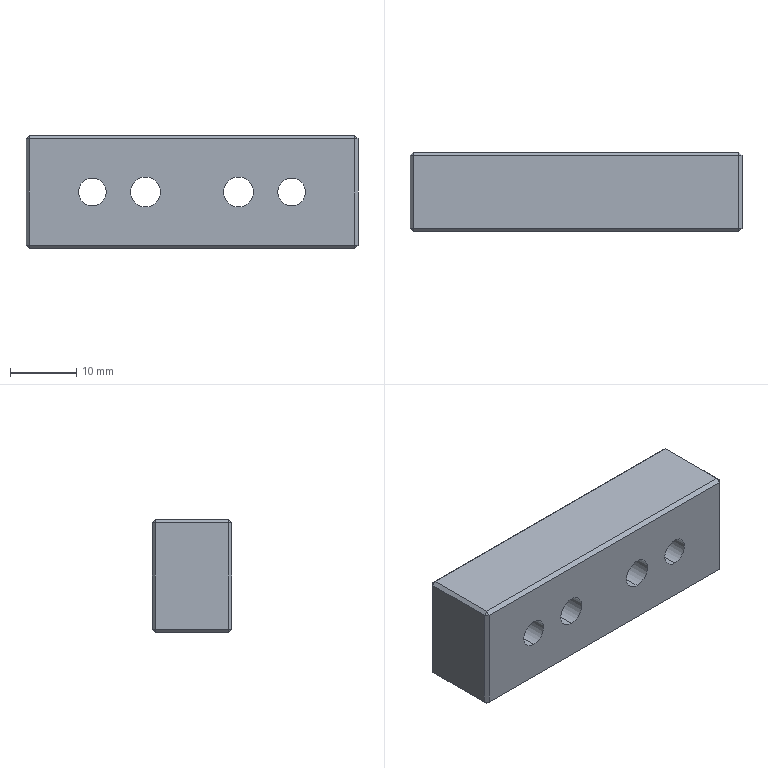Part | STEP file | H_ND24033-01-063-TL | 1 solid | 40 faces | box 50 x 12 x 17 mm | volume 9145 mm3 | plane 28 | cylinder 12 | commonest cylinder face diameters 4.2 x4 4.5 x4 8 x4